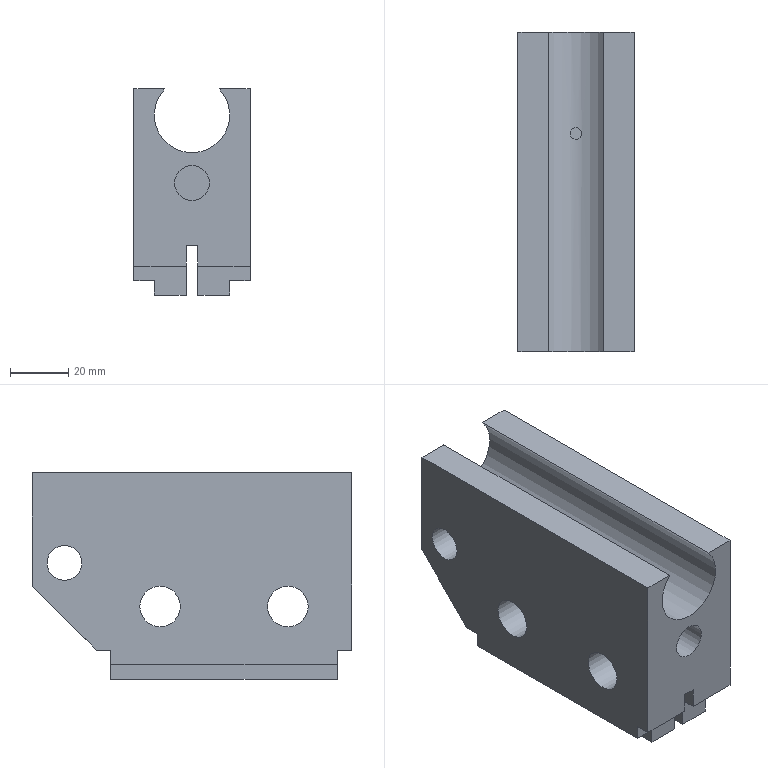Part | NX | features EXTRUDE 7, DATUM_CSYS 6, SKETCH 5 | 1 solid | 32 faces | box 40 x 110 x 71 mm | volume 205746 mm3 | plane 26 | cylinder 6 | commonest cylinder face diameters 12 x2 14 x2 4 x1 26 x1
STEP:
#1=CARTESIAN_POINT('',(9.381,0.,67.));
#2=VERTEX_POINT('',#1);
#3=CARTESIAN_POINT('',(-9.381,0.,67.));
#4=VERTEX_POINT('',#3);
#5=CARTESIAN_POINT('',(0.,0.,58.));
#6=DIRECTION('',(0.,1.,0.));
#7=DIRECTION('',(1.,0.,0.));
#8=AXIS2_PLACEMENT_3D('',#5,#6,#7);
#9=CIRCLE('',#8,13.);
#10=EDGE_CURVE('',#2,#4,#9,.T.);
#11=ORIENTED_EDGE('',*,*,#10,.T.);
#12=CARTESIAN_POINT('',(-9.381,-110.,67.));
#13=VERTEX_POINT('',#12);
#14=CARTESIAN_POINT('',(-9.381,-110.,67.));
#15=DIRECTION('',(0.,1.,0.));
#16=VECTOR('',#15,1000.);
#17=LINE('',#14,#16);
#18=EDGE_CURVE('',#13,#4,#17,.T.);
#19=ORIENTED_EDGE('',*,*,#18,.F.);
#20=CARTESIAN_POINT('',(9.381,-110.,67.));
#21=VERTEX_POINT('',#20);
#22=CARTESIAN_POINT('',(0.,-110.,58.));
#23=DIRECTION('',(0.,1.,0.));
#24=DIRECTION('',(1.,0.,0.));
#25=AXIS2_PLACEMENT_3D('',#22,#23,#24);
#26=CIRCLE('',#25,13.);
#27=EDGE_CURVE('',#21,#13,#26,.T.);
#28=ORIENTED_EDGE('',*,*,#27,.F.);
#29=CARTESIAN_POINT('',(9.381,-110.,67.));
#30=DIRECTION('',(0.,1.,0.));
#31=VECTOR('',#30,1000.);
#32=LINE('',#29,#31);
#33=EDGE_CURVE('',#21,#2,#32,.T.);
#34=ORIENTED_EDGE('',*,*,#33,.T.);
#35=EDGE_LOOP('',(#11,#19,#28,#34));
#36=FACE_BOUND('',#35,.T.);
#37=CARTESIAN_POINT('',(-2.,-34.877,45.155));
#38=VERTEX_POINT('',#37);
#39=CARTESIAN_POINT('',(-1.566,-33.308,45.077));
#40=CARTESIAN_POINT('',(-2.217,-34.877,45.194));
#41=CARTESIAN_POINT('',(-1.566,-36.444,45.077));
#42=CARTESIAN_POINT('',(-0.001886,-37.093,44.962));
#43=CARTESIAN_POINT('',(1.567,-36.444,45.077));
#44=CARTESIAN_POINT('',(2.216,-34.877,45.194));
#45=CARTESIAN_POINT('',(1.569,-33.311,45.077));
#46=CARTESIAN_POINT('',(0.001769,-32.66,44.962));
#47=CARTESIAN_POINT('',(-1.566,-33.308,45.077));
#48=CARTESIAN_POINT('',(-2.217,-34.877,45.194));
#49=CARTESIAN_POINT('',(-1.566,-36.444,45.077));
#50=B_SPLINE_CURVE_WITH_KNOTS('',3,(#39,#40,#41,#42,#43,#44,#45,#46,#47,#48,#49),.UNSPECIFIED.,.T.,.F.,(1,1,1,1,1,1,1,1,1,1,1,1,1,1,1),(-0.004696,-0.003131,-0.001565,0.,0.001565,0.003131,0.004696,0.006261,0.007827,0.009392,0.01096,0.01252,0.01409,0.01565,0.01722),.UNSPECIFIED.);
#51=EDGE_CURVE('',#38,#38,#50,.T.);
#52=ORIENTED_EDGE('',*,*,#51,.F.);
#53=EDGE_LOOP('',(#52));
#54=FACE_BOUND('',#53,.T.);
#55=CARTESIAN_POINT('',(0.,-110.,58.));
#56=DIRECTION('',(0.,1.,0.));
#57=DIRECTION('',(0.,0.,1.));
#58=AXIS2_PLACEMENT_3D('',#55,#56,#57);
#59=CYLINDRICAL_SURFACE('',#58,13.);
#60=ADVANCED_FACE('',(#36,#54),#59,.F.);
#61=CARTESIAN_POINT('',(-20.,-5.075,36.));
#62=VERTEX_POINT('',#61);
#63=CARTESIAN_POINT('',(-20.,-11.075,36.));
#64=DIRECTION('',(-1.,0.,0.));
#65=DIRECTION('',(0.,1.,0.));
#66=AXIS2_PLACEMENT_3D('',#63,#64,#65);
#67=CIRCLE('',#66,6.);
#68=EDGE_CURVE('',#62,#62,#67,.T.);
#69=ORIENTED_EDGE('',*,*,#68,.F.);
#70=EDGE_LOOP('',(#69));
#71=FACE_BOUND('',#70,.T.);
#72=CARTESIAN_POINT('',(-20.,-81.,21.));
#73=VERTEX_POINT('',#72);
#74=CARTESIAN_POINT('',(-20.,-88.,21.));
#75=DIRECTION('',(-1.,0.,0.));
#76=DIRECTION('',(0.,1.,0.));
#77=AXIS2_PLACEMENT_3D('',#74,#75,#76);
#78=CIRCLE('',#77,7.);
#79=EDGE_CURVE('',#73,#73,#78,.T.);
#80=ORIENTED_EDGE('',*,*,#79,.F.);
#81=EDGE_LOOP('',(#80));
#82=FACE_BOUND('',#81,.T.);
#83=CARTESIAN_POINT('',(-20.,-37.,21.));
#84=VERTEX_POINT('',#83);
#85=CARTESIAN_POINT('',(-20.,-44.,21.));
#86=DIRECTION('',(1.,0.,0.));
#87=DIRECTION('',(0.,1.,0.));
#88=AXIS2_PLACEMENT_3D('',#85,#86,#87);
#89=CIRCLE('',#88,7.);
#90=EDGE_CURVE('',#84,#84,#89,.T.);
#91=ORIENTED_EDGE('',*,*,#90,.T.);
#92=EDGE_LOOP('',(#91));
#93=FACE_BOUND('',#92,.T.);
#94=CARTESIAN_POINT('',(-20.,-105.007,1.));
#95=VERTEX_POINT('',#94);
#96=CARTESIAN_POINT('',(-20.,-26.993,1.));
#97=VERTEX_POINT('',#96);
#98=CARTESIAN_POINT('',(-20.,-200.,1.));
#99=DIRECTION('',(0.,1.,0.));
#100=VECTOR('',#99,1000.);
#101=LINE('',#98,#100);
#102=EDGE_CURVE('',#95,#97,#101,.T.);
#103=ORIENTED_EDGE('',*,*,#102,.F.);
#104=CARTESIAN_POINT('',(-20.,-105.007,6.));
#105=VERTEX_POINT('',#104);
#106=CARTESIAN_POINT('',(-20.,-105.007,-4.));
#107=DIRECTION('',(0.,0.,1.));
#108=VECTOR('',#107,1000.);
#109=LINE('',#106,#108);
#110=EDGE_CURVE('',#95,#105,#109,.T.);
#111=ORIENTED_EDGE('',*,*,#110,.T.);
#112=CARTESIAN_POINT('',(-20.,-110.,6.));
#113=VERTEX_POINT('',#112);
#114=CARTESIAN_POINT('',(-20.,-105.007,6.));
#115=DIRECTION('',(0.,-1.,0.));
#116=VECTOR('',#115,1000.);
#117=LINE('',#114,#116);
#118=EDGE_CURVE('',#105,#113,#117,.T.);
#119=ORIENTED_EDGE('',*,*,#118,.T.);
#120=CARTESIAN_POINT('',(-20.,-110.,67.));
#121=VERTEX_POINT('',#120);
#122=CARTESIAN_POINT('',(-20.,-110.,67.));
#123=DIRECTION('',(0.,0.,-1.));
#124=VECTOR('',#123,1000.);
#125=LINE('',#122,#124);
#126=EDGE_CURVE('',#121,#113,#125,.T.);
#127=ORIENTED_EDGE('',*,*,#126,.F.);
#128=CARTESIAN_POINT('',(-20.,0.,67.));
#129=VERTEX_POINT('',#128);
#130=CARTESIAN_POINT('',(-20.,-110.,67.));
#131=DIRECTION('',(0.,1.,0.));
#132=VECTOR('',#131,1000.);
#133=LINE('',#130,#132);
#134=EDGE_CURVE('',#121,#129,#133,.T.);
#135=ORIENTED_EDGE('',*,*,#134,.T.);
#136=CARTESIAN_POINT('',(-20.,0.,28.));
#137=VERTEX_POINT('',#136);
#138=CARTESIAN_POINT('',(-20.,0.,67.));
#139=DIRECTION('',(0.,0.,-1.));
#140=VECTOR('',#139,1000.);
#141=LINE('',#138,#140);
#142=EDGE_CURVE('',#129,#137,#141,.T.);
#143=ORIENTED_EDGE('',*,*,#142,.T.);
#144=CARTESIAN_POINT('',(-20.,-22.,6.));
#145=VERTEX_POINT('',#144);
#146=CARTESIAN_POINT('',(-20.,0.,28.));
#147=DIRECTION('',(0.,-0.7071,-0.7071));
#148=VECTOR('',#147,1000.);
#149=LINE('',#146,#148);
#150=EDGE_CURVE('',#137,#145,#149,.T.);
#151=ORIENTED_EDGE('',*,*,#150,.T.);
#152=CARTESIAN_POINT('',(-20.,-26.993,6.));
#153=VERTEX_POINT('',#152);
#154=CARTESIAN_POINT('',(-20.,-26.993,6.));
#155=DIRECTION('',(0.,1.,0.));
#156=VECTOR('',#155,1000.);
#157=LINE('',#154,#156);
#158=EDGE_CURVE('',#153,#145,#157,.T.);
#159=ORIENTED_EDGE('',*,*,#158,.F.);
#160=CARTESIAN_POINT('',(-20.,-26.993,-4.));
#161=DIRECTION('',(0.,0.,1.));
#162=VECTOR('',#161,1000.);
#163=LINE('',#160,#162);
#164=EDGE_CURVE('',#97,#153,#163,.T.);
#165=ORIENTED_EDGE('',*,*,#164,.F.);
#166=EDGE_LOOP('',(#103,#111,#119,#127,#135,#143,#151,#159,#165));
#167=FACE_BOUND('',#166,.T.);
#168=CARTESIAN_POINT('',(-20.,-110.,67.));
#169=DIRECTION('',(1.,0.,0.));
#170=DIRECTION('',(0.,0.,-1.));
#171=AXIS2_PLACEMENT_3D('',#168,#169,#170);
#172=PLANE('',#171);
#173=ADVANCED_FACE('',(#71,#82,#93,#167),#172,.F.);
#174=CARTESIAN_POINT('',(-13.,-105.007,1.));
#175=VERTEX_POINT('',#174);
#176=CARTESIAN_POINT('',(-20.,-105.007,1.));
#177=DIRECTION('',(-1.,0.,0.));
#178=VECTOR('',#177,1000.);
#179=LINE('',#176,#178);
#180=EDGE_CURVE('',#175,#95,#179,.T.);
#181=ORIENTED_EDGE('',*,*,#180,.F.);
#182=CARTESIAN_POINT('',(-13.,-105.007,-4.));
#183=VERTEX_POINT('',#182);
#184=CARTESIAN_POINT('',(-13.,-105.007,0.));
#185=DIRECTION('',(0.,0.,1.));
#186=VECTOR('',#185,1000.);
#187=LINE('',#184,#186);
#188=EDGE_CURVE('',#183,#175,#187,.T.);
#189=ORIENTED_EDGE('',*,*,#188,.F.);
#190=CARTESIAN_POINT('',(-2.,-105.007,-4.));
#191=VERTEX_POINT('',#190);
#192=CARTESIAN_POINT('',(-20.,-105.007,-4.));
#193=DIRECTION('',(1.,0.,0.));
#194=VECTOR('',#193,1000.);
#195=LINE('',#192,#194);
#196=EDGE_CURVE('',#183,#191,#195,.T.);
#197=ORIENTED_EDGE('',*,*,#196,.T.);
#198=CARTESIAN_POINT('',(-2.,-105.007,6.));
#199=VERTEX_POINT('',#198);
#200=CARTESIAN_POINT('',(-2.,-105.007,-4.));
#201=DIRECTION('',(0.,0.,-1.));
#202=VECTOR('',#201,1000.);
#203=LINE('',#200,#202);
#204=EDGE_CURVE('',#199,#191,#203,.T.);
#205=ORIENTED_EDGE('',*,*,#204,.F.);
#206=CARTESIAN_POINT('',(-20.,-105.007,6.));
#207=DIRECTION('',(1.,0.,0.));
#208=VECTOR('',#207,1000.);
#209=LINE('',#206,#208);
#210=EDGE_CURVE('',#199,#105,#209,.F.);
#211=ORIENTED_EDGE('',*,*,#210,.T.);
#212=ORIENTED_EDGE('',*,*,#110,.F.);
#213=EDGE_LOOP('',(#181,#189,#197,#205,#211,#212));
#214=FACE_BOUND('',#213,.T.);
#215=CARTESIAN_POINT('',(-20.,-105.007,-4.));
#216=DIRECTION('',(0.,1.,0.));
#217=DIRECTION('',(0.,0.,1.));
#218=AXIS2_PLACEMENT_3D('',#215,#216,#217);
#219=PLANE('',#218);
#220=ADVANCED_FACE('',(#214),#219,.F.);
#221=CARTESIAN_POINT('',(-13.,-26.993,-4.));
#222=VERTEX_POINT('',#221);
#223=CARTESIAN_POINT('',(-13.,-26.993,1.));
#224=VERTEX_POINT('',#223);
#225=CARTESIAN_POINT('',(-13.,-26.993,0.));
#226=DIRECTION('',(0.,0.,1.));
#227=VECTOR('',#226,1000.);
#228=LINE('',#225,#227);
#229=EDGE_CURVE('',#222,#224,#228,.T.);
#230=ORIENTED_EDGE('',*,*,#229,.T.);
#231=CARTESIAN_POINT('',(-20.,-26.993,1.));
#232=DIRECTION('',(-1.,0.,0.));
#233=VECTOR('',#232,1000.);
#234=LINE('',#231,#233);
#235=EDGE_CURVE('',#224,#97,#234,.T.);
#236=ORIENTED_EDGE('',*,*,#235,.T.);
#237=ORIENTED_EDGE('',*,*,#164,.T.);
#238=CARTESIAN_POINT('',(-2.,-26.993,6.));
#239=VERTEX_POINT('',#238);
#240=CARTESIAN_POINT('',(-20.,-26.993,6.));
#241=DIRECTION('',(1.,0.,0.));
#242=VECTOR('',#241,1000.);
#243=LINE('',#240,#242);
#244=EDGE_CURVE('',#239,#153,#243,.F.);
#245=ORIENTED_EDGE('',*,*,#244,.F.);
#246=CARTESIAN_POINT('',(-2.,-26.993,-4.));
#247=VERTEX_POINT('',#246);
#248=CARTESIAN_POINT('',(-2.,-26.993,-4.));
#249=DIRECTION('',(0.,0.,-1.));
#250=VECTOR('',#249,1000.);
#251=LINE('',#248,#250);
#252=EDGE_CURVE('',#239,#247,#251,.T.);
#253=ORIENTED_EDGE('',*,*,#252,.T.);
#254=CARTESIAN_POINT('',(-20.,-26.993,-4.));
#255=DIRECTION('',(1.,0.,0.));
#256=VECTOR('',#255,1000.);
#257=LINE('',#254,#256);
#258=EDGE_CURVE('',#222,#247,#257,.T.);
#259=ORIENTED_EDGE('',*,*,#258,.F.);
#260=EDGE_LOOP('',(#230,#236,#237,#245,#253,#259));
#261=FACE_BOUND('',#260,.T.);
#262=CARTESIAN_POINT('',(-20.,-26.993,-4.));
#263=DIRECTION('',(0.,1.,0.));
#264=DIRECTION('',(0.,0.,1.));
#265=AXIS2_PLACEMENT_3D('',#262,#263,#264);
#266=PLANE('',#265);
#267=ADVANCED_FACE('',(#261),#266,.T.);
#268=ORIENTED_EDGE('',*,*,#229,.F.);
#269=CARTESIAN_POINT('',(-13.,-110.,-4.));
#270=DIRECTION('',(0.,1.,0.));
#271=VECTOR('',#270,1000.);
#272=LINE('',#269,#271);
#273=EDGE_CURVE('',#183,#222,#272,.T.);
#274=ORIENTED_EDGE('',*,*,#273,.F.);
#275=ORIENTED_EDGE('',*,*,#188,.T.);
#276=CARTESIAN_POINT('',(-13.,-200.,1.));
#277=DIRECTION('',(0.,1.,0.));
#278=VECTOR('',#277,1000.);
#279=LINE('',#276,#278);
#280=EDGE_CURVE('',#175,#224,#279,.T.);
#281=ORIENTED_EDGE('',*,*,#280,.T.);
#282=EDGE_LOOP('',(#268,#274,#275,#281));
#283=FACE_BOUND('',#282,.T.);
#284=CARTESIAN_POINT('',(-13.,-110.,0.));
#285=DIRECTION('',(1.,0.,0.));
#286=DIRECTION('',(0.,0.,-1.));
#287=AXIS2_PLACEMENT_3D('',#284,#285,#286);
#288=PLANE('',#287);
#289=ADVANCED_FACE('',(#283),#288,.F.);
#290=CARTESIAN_POINT('',(-2.,-22.,6.));
#291=VERTEX_POINT('',#290);
#292=CARTESIAN_POINT('',(-2.,-110.,6.));
#293=DIRECTION('',(0.,-1.,0.));
#294=VECTOR('',#293,1000.);
#295=LINE('',#292,#294);
#296=EDGE_CURVE('',#291,#239,#295,.T.);
#297=ORIENTED_EDGE('',*,*,#296,.F.);
#298=CARTESIAN_POINT('',(-2.,-15.,13.));
#299=VERTEX_POINT('',#298);
#300=CARTESIAN_POINT('',(-2.,-71.,-43.));
#301=DIRECTION('',(0.,0.7071,0.7071));
#302=VECTOR('',#301,1000.);
#303=LINE('',#300,#302);
#304=EDGE_CURVE('',#291,#299,#303,.T.);
#305=ORIENTED_EDGE('',*,*,#304,.T.);
#306=CARTESIAN_POINT('',(-2.,-110.,13.));
#307=VERTEX_POINT('',#306);
#308=CARTESIAN_POINT('',(-2.,-110.,13.));
#309=DIRECTION('',(0.,1.,0.));
#310=VECTOR('',#309,1000.);
#311=LINE('',#308,#310);
#312=EDGE_CURVE('',#307,#299,#311,.T.);
#313=ORIENTED_EDGE('',*,*,#312,.F.);
#314=CARTESIAN_POINT('',(-2.,-110.,6.));
#315=VERTEX_POINT('',#314);
#316=CARTESIAN_POINT('',(-2.,-110.,-4.));
#317=DIRECTION('',(0.,0.,1.));
#318=VECTOR('',#317,1000.);
#319=LINE('',#316,#318);
#320=EDGE_CURVE('',#315,#307,#319,.T.);
#321=ORIENTED_EDGE('',*,*,#320,.F.);
#322=CARTESIAN_POINT('',(-2.,-110.,6.));
#323=DIRECTION('',(0.,1.,0.));
#324=VECTOR('',#323,1000.);
#325=LINE('',#322,#324);
#326=EDGE_CURVE('',#315,#199,#325,.T.);
#327=ORIENTED_EDGE('',*,*,#326,.T.);
#328=ORIENTED_EDGE('',*,*,#204,.T.);
#329=CARTESIAN_POINT('',(-2.,-110.,-4.));
#330=DIRECTION('',(0.,1.,0.));
#331=VECTOR('',#330,1000.);
#332=LINE('',#329,#331);
#333=EDGE_CURVE('',#191,#247,#332,.T.);
#334=ORIENTED_EDGE('',*,*,#333,.T.);
#335=ORIENTED_EDGE('',*,*,#252,.F.);
#336=EDGE_LOOP('',(#297,#305,#313,#321,#327,#328,#334,#335));
#337=FACE_BOUND('',#336,.T.);
#338=CARTESIAN_POINT('',(-2.,-110.,-4.));
#339=DIRECTION('',(-1.,0.,0.));
#340=DIRECTION('',(0.,0.,1.));
#341=AXIS2_PLACEMENT_3D('',#338,#339,#340);
#342=PLANE('',#341);
#343=ADVANCED_FACE('',(#337),#342,.F.);
#344=CARTESIAN_POINT('',(2.,-26.993,6.));
#345=VERTEX_POINT('',#344);
#346=CARTESIAN_POINT('',(2.,-22.,6.));
#347=VERTEX_POINT('',#346);
#348=CARTESIAN_POINT('',(2.,-110.,6.));
#349=DIRECTION('',(0.,1.,0.));
#350=VECTOR('',#349,1000.);
#351=LINE('',#348,#350);
#352=EDGE_CURVE('',#345,#347,#351,.T.);
#353=ORIENTED_EDGE('',*,*,#352,.F.);
#354=CARTESIAN_POINT('',(2.,-26.993,-4.));
#355=VERTEX_POINT('',#354);
#356=CARTESIAN_POINT('',(2.,-26.993,13.));
#357=DIRECTION('',(0.,0.,1.));
#358=VECTOR('',#357,1000.);
#359=LINE('',#356,#358);
#360=EDGE_CURVE('',#355,#345,#359,.T.);
#361=ORIENTED_EDGE('',*,*,#360,.F.);
#362=CARTESIAN_POINT('',(2.,-105.007,-4.));
#363=VERTEX_POINT('',#362);
#364=CARTESIAN_POINT('',(2.,-110.,-4.));
#365=DIRECTION('',(0.,1.,0.));
#366=VECTOR('',#365,1000.);
#367=LINE('',#364,#366);
#368=EDGE_CURVE('',#363,#355,#367,.T.);
#369=ORIENTED_EDGE('',*,*,#368,.F.);
#370=CARTESIAN_POINT('',(2.,-105.007,6.));
#371=VERTEX_POINT('',#370);
#372=CARTESIAN_POINT('',(2.,-105.007,13.));
#373=DIRECTION('',(0.,0.,1.));
#374=VECTOR('',#373,1000.);
#375=LINE('',#372,#374);
#376=EDGE_CURVE('',#363,#371,#375,.T.);
#377=ORIENTED_EDGE('',*,*,#376,.T.);
#378=CARTESIAN_POINT('',(2.,-110.,6.));
#379=VERTEX_POINT('',#378);
#380=CARTESIAN_POINT('',(2.,-110.,6.));
#381=DIRECTION('',(0.,-1.,0.));
#382=VECTOR('',#381,1000.);
#383=LINE('',#380,#382);
#384=EDGE_CURVE('',#371,#379,#383,.T.);
#385=ORIENTED_EDGE('',*,*,#384,.T.);
#386=CARTESIAN_POINT('',(2.,-110.,13.));
#387=VERTEX_POINT('',#386);
#388=CARTESIAN_POINT('',(2.,-110.,13.));
#389=DIRECTION('',(0.,0.,-1.));
#390=VECTOR('',#389,1000.);
#391=LINE('',#388,#390);
#392=EDGE_CURVE('',#387,#379,#391,.T.);
#393=ORIENTED_EDGE('',*,*,#392,.F.);
#394=CARTESIAN_POINT('',(2.,-15.,13.));
#395=VERTEX_POINT('',#394);
#396=CARTESIAN_POINT('',(2.,-110.,13.));
#397=DIRECTION('',(0.,1.,0.));
#398=VECTOR('',#397,1000.);
#399=LINE('',#396,#398);
#400=EDGE_CURVE('',#387,#395,#399,.T.);
#401=ORIENTED_EDGE('',*,*,#400,.T.);
#402=CARTESIAN_POINT('',(2.,-62.5,-34.5));
#403=DIRECTION('',(0.,-0.7071,-0.7071));
#404=VECTOR('',#403,1000.);
#405=LINE('',#402,#404);
#406=EDGE_CURVE('',#395,#347,#405,.T.);
#407=ORIENTED_EDGE('',*,*,#406,.T.);
#408=EDGE_LOOP('',(#353,#361,#369,#377,#385,#393,#401,#407));
#409=FACE_BOUND('',#408,.T.);
#410=CARTESIAN_POINT('',(2.,-110.,13.));
#411=DIRECTION('',(1.,0.,0.));
#412=DIRECTION('',(0.,0.,-1.));
#413=AXIS2_PLACEMENT_3D('',#410,#411,#412);
#414=PLANE('',#413);
#415=ADVANCED_FACE('',(#409),#414,.F.);
#416=CARTESIAN_POINT('',(13.,-26.993,1.));
#417=VERTEX_POINT('',#416);
#418=CARTESIAN_POINT('',(13.,-26.993,-4.));
#419=VERTEX_POINT('',#418);
#420=CARTESIAN_POINT('',(13.,-26.993,-4.));
#421=DIRECTION('',(0.,0.,-1.));
#422=VECTOR('',#421,1000.);
#423=LINE('',#420,#422);
#424=EDGE_CURVE('',#417,#419,#423,.T.);
#425=ORIENTED_EDGE('',*,*,#424,.F.);
#426=CARTESIAN_POINT('',(13.,-105.007,1.));
#427=VERTEX_POINT('',#426);
#428=CARTESIAN_POINT('',(13.,-200.,1.));
#429=DIRECTION('',(0.,1.,0.));
#430=VECTOR('',#429,1000.);
#431=LINE('',#428,#430);
#432=EDGE_CURVE('',#427,#417,#431,.T.);
#433=ORIENTED_EDGE('',*,*,#432,.F.);
#434=CARTESIAN_POINT('',(13.,-105.007,-4.));
#435=VERTEX_POINT('',#434);
#436=CARTESIAN_POINT('',(13.,-105.007,-4.));
#437=DIRECTION('',(0.,0.,-1.));
#438=VECTOR('',#437,1000.);
#439=LINE('',#436,#438);
#440=EDGE_CURVE('',#427,#435,#439,.T.);
#441=ORIENTED_EDGE('',*,*,#440,.T.);
#442=CARTESIAN_POINT('',(13.,-110.,-4.));
#443=DIRECTION('',(0.,1.,0.));
#444=VECTOR('',#443,1000.);
#445=LINE('',#442,#444);
#446=EDGE_CURVE('',#435,#419,#445,.T.);
#447=ORIENTED_EDGE('',*,*,#446,.T.);
#448=EDGE_LOOP('',(#425,#433,#441,#447));
#449=FACE_BOUND('',#448,.T.);
#450=CARTESIAN_POINT('',(13.,-110.,-4.));
#451=DIRECTION('',(-1.,0.,0.));
#452=DIRECTION('',(0.,0.,1.));
#453=AXIS2_PLACEMENT_3D('',#450,#451,#452);
#454=PLANE('',#453);
#455=ADVANCED_FACE('',(#449),#454,.F.);
#456=CARTESIAN_POINT('',(20.,-5.075,36.));
#457=VERTEX_POINT('',#456);
#458=CARTESIAN_POINT('',(20.,-11.075,36.));
#459=DIRECTION('',(-1.,0.,0.));
#460=DIRECTION('',(0.,1.,0.));
#461=AXIS2_PLACEMENT_3D('',#458,#459,#460);
#462=CIRCLE('',#461,6.);
#463=EDGE_CURVE('',#457,#457,#462,.T.);
#464=ORIENTED_EDGE('',*,*,#463,.T.);
#465=EDGE_LOOP('',(#464));
#466=FACE_BOUND('',#465,.T.);
#467=CARTESIAN_POINT('',(20.,-37.,21.));
#468=VERTEX_POINT('',#467);
#469=CARTESIAN_POINT('',(20.,-44.,21.));
#470=DIRECTION('',(1.,0.,0.));
#471=DIRECTION('',(0.,1.,0.));
#472=AXIS2_PLACEMENT_3D('',#469,#470,#471);
#473=CIRCLE('',#472,7.);
#474=EDGE_CURVE('',#468,#468,#473,.T.);
#475=ORIENTED_EDGE('',*,*,#474,.F.);
#476=EDGE_LOOP('',(#475));
#477=FACE_BOUND('',#476,.T.);
#478=CARTESIAN_POINT('',(20.,-81.,21.));
#479=VERTEX_POINT('',#478);
#480=CARTESIAN_POINT('',(20.,-88.,21.));
#481=DIRECTION('',(-1.,0.,0.));
#482=DIRECTION('',(0.,1.,0.));
#483=AXIS2_PLACEMENT_3D('',#480,#481,#482);
#484=CIRCLE('',#483,7.);
#485=EDGE_CURVE('',#479,#479,#484,.T.);
#486=ORIENTED_EDGE('',*,*,#485,.T.);
#487=EDGE_LOOP('',(#486));
#488=FACE_BOUND('',#487,.T.);
#489=CARTESIAN_POINT('',(20.,-105.007,1.));
#490=VERTEX_POINT('',#489);
#491=CARTESIAN_POINT('',(20.,-105.007,6.));
#492=VERTEX_POINT('',#491);
#493=CARTESIAN_POINT('',(20.,-105.007,-4.));
#494=DIRECTION('',(0.,0.,1.));
#495=VECTOR('',#494,1000.);
#496=LINE('',#493,#495);
#497=EDGE_CURVE('',#490,#492,#496,.T.);
#498=ORIENTED_EDGE('',*,*,#497,.F.);
#499=CARTESIAN_POINT('',(20.,-26.993,1.));
#500=VERTEX_POINT('',#499);
#501=CARTESIAN_POINT('',(20.,-200.,1.));
#502=DIRECTION('',(0.,1.,0.));
#503=VECTOR('',#502,1000.);
#504=LINE('',#501,#503);
#505=EDGE_CURVE('',#490,#500,#504,.T.);
#506=ORIENTED_EDGE('',*,*,#505,.T.);
#507=CARTESIAN_POINT('',(20.,-26.993,6.));
#508=VERTEX_POINT('',#507);
#509=CARTESIAN_POINT('',(20.,-26.993,-4.));
#510=DIRECTION('',(0.,0.,1.));
#511=VECTOR('',#510,1000.);
#512=LINE('',#509,#511);
#513=EDGE_CURVE('',#500,#508,#512,.T.);
#514=ORIENTED_EDGE('',*,*,#513,.T.);
#515=CARTESIAN_POINT('',(20.,-22.,6.));
#516=VERTEX_POINT('',#515);
#517=CARTESIAN_POINT('',(20.,-26.993,6.));
#518=DIRECTION('',(0.,1.,0.));
#519=VECTOR('',#518,1000.);
#520=LINE('',#517,#519);
#521=EDGE_CURVE('',#508,#516,#520,.T.);
#522=ORIENTED_EDGE('',*,*,#521,.T.);
#523=CARTESIAN_POINT('',(20.,0.,28.));
#524=VERTEX_POINT('',#523);
#525=CARTESIAN_POINT('',(20.,0.,28.));
#526=DIRECTION('',(0.,-0.7071,-0.7071));
#527=VECTOR('',#526,1000.);
#528=LINE('',#525,#527);
#529=EDGE_CURVE('',#524,#516,#528,.T.);
#530=ORIENTED_EDGE('',*,*,#529,.F.);
#531=CARTESIAN_POINT('',(20.,0.,67.));
#532=VERTEX_POINT('',#531);
#533=CARTESIAN_POINT('',(20.,0.,0.));
#534=DIRECTION('',(0.,0.,1.));
#535=VECTOR('',#534,1000.);
#536=LINE('',#533,#535);
#537=EDGE_CURVE('',#524,#532,#536,.T.);
#538=ORIENTED_EDGE('',*,*,#537,.T.);
#539=CARTESIAN_POINT('',(20.,-110.,67.));
#540=VERTEX_POINT('',#539);
#541=CARTESIAN_POINT('',(20.,-110.,67.));
#542=DIRECTION('',(0.,1.,0.));
#543=VECTOR('',#542,1000.);
#544=LINE('',#541,#543);
#545=EDGE_CURVE('',#540,#532,#544,.T.);
#546=ORIENTED_EDGE('',*,*,#545,.F.);
#547=CARTESIAN_POINT('',(20.,-110.,6.));
#548=VERTEX_POINT('',#547);
#549=CARTESIAN_POINT('',(20.,-110.,0.));
#550=DIRECTION('',(0.,0.,1.));
#551=VECTOR('',#550,1000.);
#552=LINE('',#549,#551);
#553=EDGE_CURVE('',#548,#540,#552,.T.);
#554=ORIENTED_EDGE('',*,*,#553,.F.);
#555=CARTESIAN_POINT('',(20.,-105.007,6.));
#556=DIRECTION('',(0.,-1.,0.));
#557=VECTOR('',#556,1000.);
#558=LINE('',#555,#557);
#559=EDGE_CURVE('',#492,#548,#558,.T.);
#560=ORIENTED_EDGE('',*,*,#559,.F.);
#561=EDGE_LOOP('',(#498,#506,#514,#522,#530,#538,#546,#554,#560));
#562=FACE_BOUND('',#561,.T.);
#563=CARTESIAN_POINT('',(20.,-110.,0.));
#564=DIRECTION('',(-1.,0.,0.));
#565=DIRECTION('',(0.,0.,1.));
#566=AXIS2_PLACEMENT_3D('',#563,#564,#565);
#567=PLANE('',#566);
#568=ADVANCED_FACE('',(#466,#477,#488,#562),#567,.F.);
#569=ORIENTED_EDGE('',*,*,#273,.T.);
#570=ORIENTED_EDGE('',*,*,#258,.T.);
#571=ORIENTED_EDGE('',*,*,#333,.F.);
#572=ORIENTED_EDGE('',*,*,#196,.F.);
#573=EDGE_LOOP('',(#569,#570,#571,#572));
#574=FACE_BOUND('',#573,.T.);
#575=CARTESIAN_POINT('',(-13.,-110.,-4.));
#576=DIRECTION('',(0.,0.,1.));
#577=DIRECTION('',(1.,0.,0.));
#578=AXIS2_PLACEMENT_3D('',#575,#576,#577);
#579=PLANE('',#578);
#580=ADVANCED_FACE('',(#574),#579,.F.);
#581=ORIENTED_EDGE('',*,*,#368,.T.);
#582=CARTESIAN_POINT('',(-20.,-26.993,-4.));
#583=DIRECTION('',(1.,0.,0.));
#584=VECTOR('',#583,1000.);
#585=LINE('',#582,#584);
#586=EDGE_CURVE('',#355,#419,#585,.T.);
#587=ORIENTED_EDGE('',*,*,#586,.T.);
#588=ORIENTED_EDGE('',*,*,#446,.F.);
#589=CARTESIAN_POINT('',(-20.,-105.007,-4.));
#590=DIRECTION('',(1.,0.,0.));
#591=VECTOR('',#590,1000.);
#592=LINE('',#589,#591);
#593=EDGE_CURVE('',#363,#435,#592,.T.);
#594=ORIENTED_EDGE('',*,*,#593,.F.);
#595=EDGE_LOOP('',(#581,#587,#588,#594));
#596=FACE_BOUND('',#595,.T.);
#597=CARTESIAN_POINT('',(2.,-110.,-4.));
#598=DIRECTION('',(0.,0.,1.));
#599=DIRECTION('',(1.,0.,0.));
#600=AXIS2_PLACEMENT_3D('',#597,#598,#599);
#601=PLANE('',#600);
#602=ADVANCED_FACE('',(#596),#601,.F.);
#603=ORIENTED_EDGE('',*,*,#312,.T.);
#604=CARTESIAN_POINT('',(-2.,-15.,13.));
#605=DIRECTION('',(1.,0.,0.));
#606=VECTOR('',#605,1000.);
#607=LINE('',#604,#606);
#608=EDGE_CURVE('',#299,#395,#607,.T.);
#609=ORIENTED_EDGE('',*,*,#608,.T.);
#610=ORIENTED_EDGE('',*,*,#400,.F.);
#611=CARTESIAN_POINT('',(-2.,-110.,13.));
#612=DIRECTION('',(1.,0.,0.));
#613=VECTOR('',#612,1000.);
#614=LINE('',#611,#613);
#615=EDGE_CURVE('',#307,#387,#614,.T.);
#616=ORIENTED_EDGE('',*,*,#615,.F.);
#617=EDGE_LOOP('',(#603,#609,#610,#616));
#618=FACE_BOUND('',#617,.T.);
#619=CARTESIAN_POINT('',(-2.,-110.,13.));
#620=DIRECTION('',(0.,0.,1.));
#621=DIRECTION('',(1.,0.,0.));
#622=AXIS2_PLACEMENT_3D('',#619,#620,#621);
#623=PLANE('',#622);
#624=ADVANCED_FACE('',(#618),#623,.F.);
#625=CARTESIAN_POINT('',(20.,0.,67.));
#626=DIRECTION('',(-1.,0.,0.));
#627=VECTOR('',#626,1000.);
#628=LINE('',#625,#627);
#629=EDGE_CURVE('',#532,#2,#628,.T.);
#630=ORIENTED_EDGE('',*,*,#629,.T.);
#631=ORIENTED_EDGE('',*,*,#33,.F.);
#632=CARTESIAN_POINT('',(20.,-110.,67.));
#633=DIRECTION('',(-1.,0.,0.));
#634=VECTOR('',#633,1000.);
#635=LINE('',#632,#634);
#636=EDGE_CURVE('',#540,#21,#635,.T.);
#637=ORIENTED_EDGE('',*,*,#636,.F.);
#638=ORIENTED_EDGE('',*,*,#545,.T.);
#639=EDGE_LOOP('',(#630,#631,#637,#638));
#640=FACE_BOUND('',#639,.T.);
#641=CARTESIAN_POINT('',(20.,-110.,67.));
#642=DIRECTION('',(0.,0.,-1.));
#643=DIRECTION('',(-1.,0.,0.));
#644=AXIS2_PLACEMENT_3D('',#641,#642,#643);
#645=PLANE('',#644);
#646=ADVANCED_FACE('',(#640),#645,.F.);
#647=CARTESIAN_POINT('',(-9.381,0.,67.));
#648=DIRECTION('',(-1.,0.,0.));
#649=VECTOR('',#648,1000.);
#650=LINE('',#647,#649);
#651=EDGE_CURVE('',#4,#129,#650,.T.);
#652=ORIENTED_EDGE('',*,*,#651,.T.);
#653=ORIENTED_EDGE('',*,*,#134,.F.);
#654=CARTESIAN_POINT('',(-9.381,-110.,67.));
#655=DIRECTION('',(-1.,0.,0.));
#656=VECTOR('',#655,1000.);
#657=LINE('',#654,#656);
#658=EDGE_CURVE('',#13,#121,#657,.T.);
#659=ORIENTED_EDGE('',*,*,#658,.F.);
#660=ORIENTED_EDGE('',*,*,#18,.T.);
#661=EDGE_LOOP('',(#652,#653,#659,#660));
#662=FACE_BOUND('',#661,.T.);
#663=CARTESIAN_POINT('',(-9.381,-110.,67.));
#664=DIRECTION('',(0.,0.,-1.));
#665=DIRECTION('',(-1.,0.,0.));
#666=AXIS2_PLACEMENT_3D('',#663,#664,#665);
#667=PLANE('',#666);
#668=ADVANCED_FACE('',(#662),#667,.F.);
#669=CARTESIAN_POINT('',(6.,-110.,34.594));
#670=VERTEX_POINT('',#669);
#671=CARTESIAN_POINT('',(0.,-110.,34.594));
#672=DIRECTION('',(0.,1.,0.));
#673=DIRECTION('',(1.,0.,0.));
#674=AXIS2_PLACEMENT_3D('',#671,#672,#673);
#675=CIRCLE('',#674,6.);
#676=EDGE_CURVE('',#670,#670,#675,.T.);
#677=ORIENTED_EDGE('',*,*,#676,.T.);
#678=EDGE_LOOP('',(#677));
#679=FACE_BOUND('',#678,.T.);
#680=ORIENTED_EDGE('',*,*,#126,.T.);
#681=CARTESIAN_POINT('',(-20.,-110.,6.));
#682=DIRECTION('',(1.,0.,0.));
#683=VECTOR('',#682,1000.);
#684=LINE('',#681,#683);
#685=EDGE_CURVE('',#113,#315,#684,.T.);
#686=ORIENTED_EDGE('',*,*,#685,.T.);
#687=ORIENTED_EDGE('',*,*,#320,.T.);
#688=ORIENTED_EDGE('',*,*,#615,.T.);
#689=ORIENTED_EDGE('',*,*,#392,.T.);
#690=CARTESIAN_POINT('',(-20.,-110.,6.));
#691=DIRECTION('',(1.,0.,0.));
#692=VECTOR('',#691,1000.);
#693=LINE('',#690,#692);
#694=EDGE_CURVE('',#379,#548,#693,.T.);
#695=ORIENTED_EDGE('',*,*,#694,.T.);
#696=ORIENTED_EDGE('',*,*,#553,.T.);
#697=ORIENTED_EDGE('',*,*,#636,.T.);
#698=ORIENTED_EDGE('',*,*,#27,.T.);
#699=ORIENTED_EDGE('',*,*,#658,.T.);
#700=EDGE_LOOP('',(#680,#686,#687,#688,#689,#695,#696,#697,#698,#699));
#701=FACE_BOUND('',#700,.T.);
#702=CARTESIAN_POINT('',(0.,-110.,58.));
#703=DIRECTION('',(0.,1.,0.));
#704=DIRECTION('',(0.,0.,1.));
#705=AXIS2_PLACEMENT_3D('',#702,#703,#704);
#706=PLANE('',#705);
#707=ADVANCED_FACE('',(#679,#701),#706,.F.);
#708=CARTESIAN_POINT('',(-20.,0.,28.));
#709=DIRECTION('',(1.,0.,0.));
#710=VECTOR('',#709,1000.);
#711=LINE('',#708,#710);
#712=EDGE_CURVE('',#137,#524,#711,.T.);
#713=ORIENTED_EDGE('',*,*,#712,.F.);
#714=ORIENTED_EDGE('',*,*,#142,.F.);
#715=ORIENTED_EDGE('',*,*,#651,.F.);
#716=ORIENTED_EDGE('',*,*,#10,.F.);
#717=ORIENTED_EDGE('',*,*,#629,.F.);
#718=ORIENTED_EDGE('',*,*,#537,.F.);
#719=EDGE_LOOP('',(#713,#714,#715,#716,#717,#718));
#720=FACE_BOUND('',#719,.T.);
#721=CARTESIAN_POINT('',(0.,0.,58.));
#722=DIRECTION('',(0.,1.,0.));
#723=DIRECTION('',(0.,0.,1.));
#724=AXIS2_PLACEMENT_3D('',#721,#722,#723);
#725=PLANE('',#724);
#726=ADVANCED_FACE('',(#720),#725,.T.);
#727=ORIENTED_EDGE('',*,*,#676,.F.);
#728=EDGE_LOOP('',(#727));
#729=FACE_BOUND('',#728,.T.);
#730=CARTESIAN_POINT('',(6.,-80.,34.594));
#731=VERTEX_POINT('',#730);
#732=CARTESIAN_POINT('',(0.,-80.,34.594));
#733=DIRECTION('',(0.,1.,0.));
#734=DIRECTION('',(1.,0.,0.));
#735=AXIS2_PLACEMENT_3D('',#732,#733,#734);
#736=CIRCLE('',#735,6.);
#737=EDGE_CURVE('',#731,#731,#736,.F.);
#738=ORIENTED_EDGE('',*,*,#737,.F.);
#739=EDGE_LOOP('',(#738));
#740=FACE_BOUND('',#739,.T.);
#741=CARTESIAN_POINT('',(0.,-110.,34.594));
#742=DIRECTION('',(0.,1.,0.));
#743=DIRECTION('',(0.,0.,1.));
#744=AXIS2_PLACEMENT_3D('',#741,#742,#743);
#745=CYLINDRICAL_SURFACE('',#744,6.);
#746=ADVANCED_FACE('',(#729,#740),#745,.F.);
#747=ORIENTED_EDGE('',*,*,#737,.T.);
#748=EDGE_LOOP('',(#747));
#749=FACE_BOUND('',#748,.T.);
#750=CARTESIAN_POINT('',(0.,-80.,34.594));
#751=DIRECTION('',(0.,1.,0.));
#752=DIRECTION('',(0.,0.,1.));
#753=AXIS2_PLACEMENT_3D('',#750,#751,#752);
#754=PLANE('',#753);
#755=ADVANCED_FACE('',(#749),#754,.F.);
#756=CARTESIAN_POINT('',(-20.,-22.,6.));
#757=DIRECTION('',(1.,0.,0.));
#758=VECTOR('',#757,1000.);
#759=LINE('',#756,#758);
#760=EDGE_CURVE('',#291,#145,#759,.F.);
#761=ORIENTED_EDGE('',*,*,#760,.T.);
#762=ORIENTED_EDGE('',*,*,#150,.F.);
#763=ORIENTED_EDGE('',*,*,#712,.T.);
#764=ORIENTED_EDGE('',*,*,#529,.T.);
#765=CARTESIAN_POINT('',(-20.,-22.,6.));
#766=DIRECTION('',(1.,0.,0.));
#767=VECTOR('',#766,1000.);
#768=LINE('',#765,#767);
#769=EDGE_CURVE('',#516,#347,#768,.F.);
#770=ORIENTED_EDGE('',*,*,#769,.T.);
#771=ORIENTED_EDGE('',*,*,#406,.F.);
#772=ORIENTED_EDGE('',*,*,#608,.F.);
#773=ORIENTED_EDGE('',*,*,#304,.F.);
#774=EDGE_LOOP('',(#761,#762,#763,#764,#770,#771,#772,#773));
#775=FACE_BOUND('',#774,.T.);
#776=CARTESIAN_POINT('',(-20.,0.,28.));
#777=DIRECTION('',(0.,-0.7071,0.7071));
#778=DIRECTION('',(0.,-0.7071,-0.7071));
#779=AXIS2_PLACEMENT_3D('',#776,#777,#778);
#780=PLANE('',#779);
#781=ADVANCED_FACE('',(#775),#780,.F.);
#782=ORIENTED_EDGE('',*,*,#90,.F.);
#783=EDGE_LOOP('',(#782));
#784=FACE_BOUND('',#783,.T.);
#785=ORIENTED_EDGE('',*,*,#474,.T.);
#786=EDGE_LOOP('',(#785));
#787=FACE_BOUND('',#786,.T.);
#788=CARTESIAN_POINT('',(-20.,-44.,21.));
#789=DIRECTION('',(1.,0.,0.));
#790=DIRECTION('',(0.,0.,-1.));
#791=AXIS2_PLACEMENT_3D('',#788,#789,#790);
#792=CYLINDRICAL_SURFACE('',#791,7.);
#793=ADVANCED_FACE('',(#784,#787),#792,.F.);
#794=ORIENTED_EDGE('',*,*,#79,.T.);
#795=EDGE_LOOP('',(#794));
#796=FACE_BOUND('',#795,.T.);
#797=ORIENTED_EDGE('',*,*,#485,.F.);
#798=EDGE_LOOP('',(#797));
#799=FACE_BOUND('',#798,.T.);
#800=CARTESIAN_POINT('',(-20.,-88.,21.));
#801=DIRECTION('',(1.,0.,0.));
#802=DIRECTION('',(0.,0.,-1.));
#803=AXIS2_PLACEMENT_3D('',#800,#801,#802);
#804=CYLINDRICAL_SURFACE('',#803,7.);
#805=ADVANCED_FACE('',(#796,#799),#804,.F.);
#806=ORIENTED_EDGE('',*,*,#440,.F.);
#807=CARTESIAN_POINT('',(-20.,-105.007,1.));
#808=DIRECTION('',(1.,0.,0.));
#809=VECTOR('',#808,1000.);
#810=LINE('',#807,#809);
#811=EDGE_CURVE('',#427,#490,#810,.T.);
#812=ORIENTED_EDGE('',*,*,#811,.T.);
#813=ORIENTED_EDGE('',*,*,#497,.T.);
#814=CARTESIAN_POINT('',(-20.,-105.007,6.));
#815=DIRECTION('',(1.,0.,0.));
#816=VECTOR('',#815,1000.);
#817=LINE('',#814,#816);
#818=EDGE_CURVE('',#492,#371,#817,.F.);
#819=ORIENTED_EDGE('',*,*,#818,.T.);
#820=ORIENTED_EDGE('',*,*,#376,.F.);
#821=ORIENTED_EDGE('',*,*,#593,.T.);
#822=EDGE_LOOP('',(#806,#812,#813,#819,#820,#821));
#823=FACE_BOUND('',#822,.T.);
#824=CARTESIAN_POINT('',(-20.,-105.007,-4.));
#825=DIRECTION('',(0.,1.,0.));
#826=DIRECTION('',(0.,0.,1.));
#827=AXIS2_PLACEMENT_3D('',#824,#825,#826);
#828=PLANE('',#827);
#829=ADVANCED_FACE('',(#823),#828,.F.);
#830=ORIENTED_EDGE('',*,*,#818,.F.);
#831=ORIENTED_EDGE('',*,*,#559,.T.);
#832=ORIENTED_EDGE('',*,*,#694,.F.);
#833=ORIENTED_EDGE('',*,*,#384,.F.);
#834=EDGE_LOOP('',(#830,#831,#832,#833));
#835=FACE_BOUND('',#834,.T.);
#836=CARTESIAN_POINT('',(-20.,-105.007,6.));
#837=DIRECTION('',(0.,0.,1.));
#838=DIRECTION('',(0.,-1.,0.));
#839=AXIS2_PLACEMENT_3D('',#836,#837,#838);
#840=PLANE('',#839);
#841=ADVANCED_FACE('',(#835),#840,.F.);
#842=ORIENTED_EDGE('',*,*,#685,.F.);
#843=ORIENTED_EDGE('',*,*,#118,.F.);
#844=ORIENTED_EDGE('',*,*,#210,.F.);
#845=ORIENTED_EDGE('',*,*,#326,.F.);
#846=EDGE_LOOP('',(#842,#843,#844,#845));
#847=FACE_BOUND('',#846,.T.);
#848=CARTESIAN_POINT('',(-20.,-105.007,6.));
#849=DIRECTION('',(0.,0.,1.));
#850=DIRECTION('',(0.,-1.,0.));
#851=AXIS2_PLACEMENT_3D('',#848,#849,#850);
#852=PLANE('',#851);
#853=ADVANCED_FACE('',(#847),#852,.F.);
#854=CARTESIAN_POINT('',(-20.,-26.993,1.));
#855=DIRECTION('',(1.,0.,0.));
#856=VECTOR('',#855,1000.);
#857=LINE('',#854,#856);
#858=EDGE_CURVE('',#417,#500,#857,.T.);
#859=ORIENTED_EDGE('',*,*,#858,.F.);
#860=ORIENTED_EDGE('',*,*,#424,.T.);
#861=ORIENTED_EDGE('',*,*,#586,.F.);
#862=ORIENTED_EDGE('',*,*,#360,.T.);
#863=CARTESIAN_POINT('',(-20.,-26.993,6.));
#864=DIRECTION('',(1.,0.,0.));
#865=VECTOR('',#864,1000.);
#866=LINE('',#863,#865);
#867=EDGE_CURVE('',#508,#345,#866,.F.);
#868=ORIENTED_EDGE('',*,*,#867,.F.);
#869=ORIENTED_EDGE('',*,*,#513,.F.);
#870=EDGE_LOOP('',(#859,#860,#861,#862,#868,#869));
#871=FACE_BOUND('',#870,.T.);
#872=CARTESIAN_POINT('',(-20.,-26.993,-4.));
#873=DIRECTION('',(0.,1.,0.));
#874=DIRECTION('',(0.,0.,1.));
#875=AXIS2_PLACEMENT_3D('',#872,#873,#874);
#876=PLANE('',#875);
#877=ADVANCED_FACE('',(#871),#876,.T.);
#878=ORIENTED_EDGE('',*,*,#352,.T.);
#879=ORIENTED_EDGE('',*,*,#769,.F.);
#880=ORIENTED_EDGE('',*,*,#521,.F.);
#881=ORIENTED_EDGE('',*,*,#867,.T.);
#882=EDGE_LOOP('',(#878,#879,#880,#881));
#883=FACE_BOUND('',#882,.T.);
#884=CARTESIAN_POINT('',(-20.,-26.993,6.));
#885=DIRECTION('',(0.,0.,-1.));
#886=DIRECTION('',(-1.,0.,0.));
#887=AXIS2_PLACEMENT_3D('',#884,#885,#886);
#888=PLANE('',#887);
#889=ADVANCED_FACE('',(#883),#888,.T.);
#890=ORIENTED_EDGE('',*,*,#296,.T.);
#891=ORIENTED_EDGE('',*,*,#244,.T.);
#892=ORIENTED_EDGE('',*,*,#158,.T.);
#893=ORIENTED_EDGE('',*,*,#760,.F.);
#894=EDGE_LOOP('',(#890,#891,#892,#893));
#895=FACE_BOUND('',#894,.T.);
#896=CARTESIAN_POINT('',(-20.,-26.993,6.));
#897=DIRECTION('',(0.,0.,-1.));
#898=DIRECTION('',(-1.,0.,0.));
#899=AXIS2_PLACEMENT_3D('',#896,#897,#898);
#900=PLANE('',#899);
#901=ADVANCED_FACE('',(#895),#900,.T.);
#902=ORIENTED_EDGE('',*,*,#432,.T.);
#903=ORIENTED_EDGE('',*,*,#858,.T.);
#904=ORIENTED_EDGE('',*,*,#505,.F.);
#905=ORIENTED_EDGE('',*,*,#811,.F.);
#906=EDGE_LOOP('',(#902,#903,#904,#905));
#907=FACE_BOUND('',#906,.T.);
#908=CARTESIAN_POINT('',(13.,-200.,1.));
#909=DIRECTION('',(0.,0.,1.));
#910=DIRECTION('',(1.,0.,0.));
#911=AXIS2_PLACEMENT_3D('',#908,#909,#910);
#912=PLANE('',#911);
#913=ADVANCED_FACE('',(#907),#912,.F.);
#914=ORIENTED_EDGE('',*,*,#180,.T.);
#915=ORIENTED_EDGE('',*,*,#102,.T.);
#916=ORIENTED_EDGE('',*,*,#235,.F.);
#917=ORIENTED_EDGE('',*,*,#280,.F.);
#918=EDGE_LOOP('',(#914,#915,#916,#917));
#919=FACE_BOUND('',#918,.T.);
#920=CARTESIAN_POINT('',(-13.,-200.,1.));
#921=DIRECTION('',(0.,0.,-1.));
#922=DIRECTION('',(-1.,0.,0.));
#923=AXIS2_PLACEMENT_3D('',#920,#921,#922);
#924=PLANE('',#923);
#925=ADVANCED_FACE('',(#919),#924,.T.);
#926=CARTESIAN_POINT('',(2.,-34.877,37.));
#927=VERTEX_POINT('',#926);
#928=CARTESIAN_POINT('',(0.,-34.877,37.));
#929=DIRECTION('',(0.,0.,1.));
#930=DIRECTION('',(1.,0.,0.));
#931=AXIS2_PLACEMENT_3D('',#928,#929,#930);
#932=CIRCLE('',#931,2.);
#933=EDGE_CURVE('',#927,#927,#932,.F.);
#934=ORIENTED_EDGE('',*,*,#933,.T.);
#935=EDGE_LOOP('',(#934));
#936=FACE_BOUND('',#935,.T.);
#937=ORIENTED_EDGE('',*,*,#51,.T.);
#938=EDGE_LOOP('',(#937));
#939=FACE_BOUND('',#938,.T.);
#940=CARTESIAN_POINT('',(0.,-34.877,47.));
#941=DIRECTION('',(0.,0.,-1.));
#942=DIRECTION('',(-1.,0.,0.));
#943=AXIS2_PLACEMENT_3D('',#940,#941,#942);
#944=CYLINDRICAL_SURFACE('',#943,2.);
#945=ADVANCED_FACE('',(#936,#939),#944,.F.);
#946=ORIENTED_EDGE('',*,*,#933,.F.);
#947=EDGE_LOOP('',(#946));
#948=FACE_BOUND('',#947,.T.);
#949=CARTESIAN_POINT('',(0.,-34.877,37.));
#950=DIRECTION('',(0.,0.,1.));
#951=DIRECTION('',(1.,0.,0.));
#952=AXIS2_PLACEMENT_3D('',#949,#950,#951);
#953=PLANE('',#952);
#954=ADVANCED_FACE('',(#948),#953,.T.);
#955=ORIENTED_EDGE('',*,*,#68,.T.);
#956=EDGE_LOOP('',(#955));
#957=FACE_BOUND('',#956,.T.);
#958=ORIENTED_EDGE('',*,*,#463,.F.);
#959=EDGE_LOOP('',(#958));
#960=FACE_BOUND('',#959,.T.);
#961=CARTESIAN_POINT('',(-20.,-11.075,36.));
#962=DIRECTION('',(1.,0.,0.));
#963=DIRECTION('',(0.,0.,-1.));
#964=AXIS2_PLACEMENT_3D('',#961,#962,#963);
#965=CYLINDRICAL_SURFACE('',#964,6.);
#966=ADVANCED_FACE('',(#957,#960),#965,.F.);
#967=CLOSED_SHELL('',(#60,#173,#220,#267,#289,#343,#415,#455,#568,#580,#602,#624,#646,#668,#707,#726,#746,#755,#781,#793,#805,#829,#841,#853,#877,#889,#901,#913,#925,#945,#954,#966));
#968=MANIFOLD_SOLID_BREP('',#967);
#969=(LENGTH_UNIT()NAMED_UNIT(*)SI_UNIT(.MILLI.,.METRE.));
#970=UNCERTAINTY_MEASURE_WITH_UNIT(LENGTH_MEASURE(0.0508),#969,'','');
#971=(NAMED_UNIT(*)PLANE_ANGLE_UNIT()SI_UNIT($,.RADIAN.));
#972=(NAMED_UNIT(*)SI_UNIT($,.STERADIAN.)SOLID_ANGLE_UNIT());
#973=(GEOMETRIC_REPRESENTATION_CONTEXT(3)GLOBAL_UNCERTAINTY_ASSIGNED_CONTEXT((#970))GLOBAL_UNIT_ASSIGNED_CONTEXT((#969,#971,#972))REPRESENTATION_CONTEXT('',''));
#974=ADVANCED_BREP_SHAPE_REPRESENTATION('',(#968),#973);